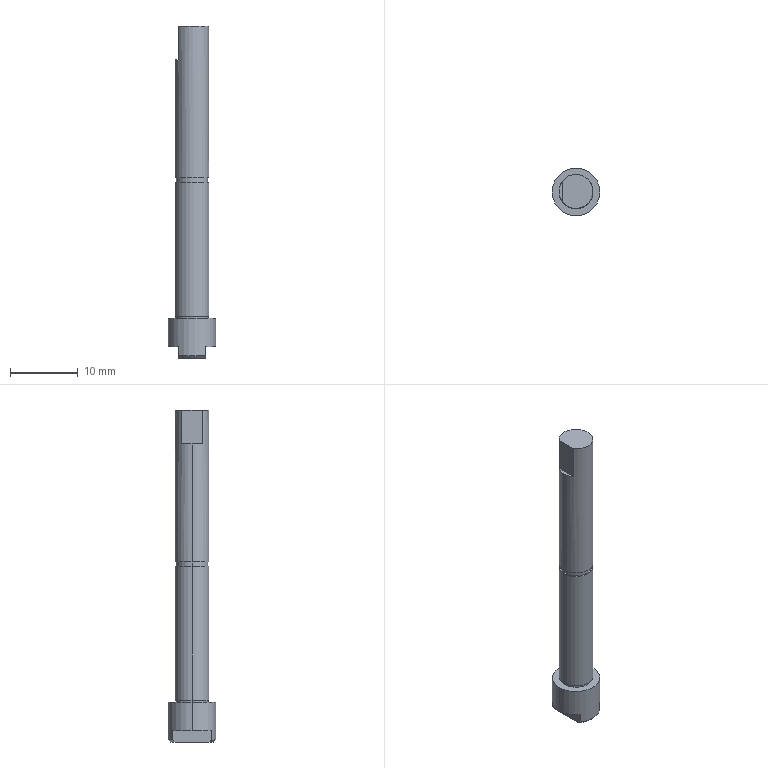Part | NX | 1 solid | 30 faces | box 7 x 7 x 48.83 mm | volume 994.875 mm3 | plane 12 | cylinder 12 | cone 6 | commonest cylinder face diameters 5 x4 2.5 x2 4.6 x2 4.8 x2 7 x2
STEP:
#1=CARTESIAN_POINT('',(-2.,1.5,43.));
#2=VERTEX_POINT('',#1);
#3=CARTESIAN_POINT('',(-2.,-1.5,43.));
#4=VERTEX_POINT('',#3);
#5=CARTESIAN_POINT('',(-2.,1.5,43.));
#6=DIRECTION('',(0.,-1.,0.));
#7=VECTOR('',#6,1000.);
#8=LINE('',#5,#7);
#9=EDGE_CURVE('',#2,#4,#8,.T.);
#10=ORIENTED_EDGE('',*,*,#9,.T.);
#11=CARTESIAN_POINT('',(2.5,0.,43.));
#12=VERTEX_POINT('',#11);
#13=CARTESIAN_POINT('',(0.,0.,43.));
#14=DIRECTION('',(0.,0.,-1.));
#15=DIRECTION('',(1.,0.,0.));
#16=AXIS2_PLACEMENT_3D('',#13,#14,#15);
#17=CIRCLE('',#16,2.5);
#18=EDGE_CURVE('',#12,#4,#17,.T.);
#19=ORIENTED_EDGE('',*,*,#18,.F.);
#20=CARTESIAN_POINT('',(0.,0.,43.));
#21=DIRECTION('',(0.,0.,-1.));
#22=DIRECTION('',(1.,0.,0.));
#23=AXIS2_PLACEMENT_3D('',#20,#21,#22);
#24=CIRCLE('',#23,2.5);
#25=EDGE_CURVE('',#2,#12,#24,.T.);
#26=ORIENTED_EDGE('',*,*,#25,.F.);
#27=EDGE_LOOP('',(#10,#19,#26));
#28=FACE_BOUND('',#27,.T.);
#29=CARTESIAN_POINT('',(0.,0.,43.));
#30=DIRECTION('',(0.,0.,1.));
#31=DIRECTION('',(1.,0.,0.));
#32=AXIS2_PLACEMENT_3D('',#29,#30,#31);
#33=PLANE('',#32);
#34=ADVANCED_FACE('',(#28),#33,.T.);
#35=ORIENTED_EDGE('',*,*,#9,.F.);
#36=CARTESIAN_POINT('',(-2.,1.5,38.));
#37=VERTEX_POINT('',#36);
#38=CARTESIAN_POINT('',(-2.,1.5,43.));
#39=DIRECTION('',(0.,0.,-1.));
#40=VECTOR('',#39,1000.);
#41=LINE('',#38,#40);
#42=EDGE_CURVE('',#2,#37,#41,.T.);
#43=ORIENTED_EDGE('',*,*,#42,.T.);
#44=CARTESIAN_POINT('',(-2.,-1.5,38.));
#45=VERTEX_POINT('',#44);
#46=CARTESIAN_POINT('',(-2.,1.5,38.));
#47=DIRECTION('',(0.,-1.,0.));
#48=VECTOR('',#47,1000.);
#49=LINE('',#46,#48);
#50=EDGE_CURVE('',#37,#45,#49,.T.);
#51=ORIENTED_EDGE('',*,*,#50,.T.);
#52=CARTESIAN_POINT('',(-2.,-1.5,38.));
#53=DIRECTION('',(0.,0.,1.));
#54=VECTOR('',#53,1000.);
#55=LINE('',#52,#54);
#56=EDGE_CURVE('',#45,#4,#55,.T.);
#57=ORIENTED_EDGE('',*,*,#56,.T.);
#58=EDGE_LOOP('',(#35,#43,#51,#57));
#59=FACE_BOUND('',#58,.T.);
#60=CARTESIAN_POINT('',(-2.,-3.316,43.));
#61=DIRECTION('',(1.,0.,0.));
#62=DIRECTION('',(0.,1.,0.));
#63=AXIS2_PLACEMENT_3D('',#60,#61,#62);
#64=PLANE('',#63);
#65=ADVANCED_FACE('',(#59),#64,.F.);
#66=CARTESIAN_POINT('',(-2.5,0.,38.));
#67=VERTEX_POINT('',#66);
#68=CARTESIAN_POINT('',(0.,0.,38.));
#69=DIRECTION('',(0.,0.,-1.));
#70=DIRECTION('',(-0.8,-0.6,0.));
#71=AXIS2_PLACEMENT_3D('',#68,#69,#70);
#72=CIRCLE('',#71,2.5);
#73=EDGE_CURVE('',#67,#37,#72,.T.);
#74=ORIENTED_EDGE('',*,*,#73,.T.);
#75=ORIENTED_EDGE('',*,*,#42,.F.);
#76=ORIENTED_EDGE('',*,*,#25,.T.);
#77=CARTESIAN_POINT('',(2.5,0.,20.65));
#78=VERTEX_POINT('',#77);
#79=CARTESIAN_POINT('',(2.5,0.,0.));
#80=DIRECTION('',(0.,0.,1.));
#81=VECTOR('',#80,1000.);
#82=LINE('',#79,#81);
#83=EDGE_CURVE('',#78,#12,#82,.T.);
#84=ORIENTED_EDGE('',*,*,#83,.F.);
#85=CARTESIAN_POINT('',(-2.5,0.,20.65));
#86=VERTEX_POINT('',#85);
#87=CARTESIAN_POINT('',(0.,0.,20.65));
#88=DIRECTION('',(0.,0.,1.));
#89=DIRECTION('',(1.,0.,0.));
#90=AXIS2_PLACEMENT_3D('',#87,#88,#89);
#91=CIRCLE('',#90,2.5);
#92=EDGE_CURVE('',#78,#86,#91,.T.);
#93=ORIENTED_EDGE('',*,*,#92,.T.);
#94=CARTESIAN_POINT('',(-2.5,0.,0.));
#95=DIRECTION('',(0.,0.,1.));
#96=VECTOR('',#95,1000.);
#97=LINE('',#94,#96);
#98=EDGE_CURVE('',#86,#67,#97,.T.);
#99=ORIENTED_EDGE('',*,*,#98,.T.);
#100=EDGE_LOOP('',(#74,#75,#76,#84,#93,#99));
#101=FACE_BOUND('',#100,.T.);
#102=CARTESIAN_POINT('',(0.,0.,0.));
#103=DIRECTION('',(0.,0.,1.));
#104=DIRECTION('',(1.,0.,0.));
#105=AXIS2_PLACEMENT_3D('',#102,#103,#104);
#106=CYLINDRICAL_SURFACE('',#105,2.5);
#107=ADVANCED_FACE('',(#101),#106,.T.);
#108=CARTESIAN_POINT('',(-2.,-2.498,-5.83));
#109=VERTEX_POINT('',#108);
#110=CARTESIAN_POINT('',(2.,-2.498,-5.83));
#111=VERTEX_POINT('',#110);
#112=CARTESIAN_POINT('',(0.,0.,-5.83));
#113=DIRECTION('',(0.,0.,1.));
#114=DIRECTION('',(1.,0.,0.));
#115=AXIS2_PLACEMENT_3D('',#112,#113,#114);
#116=CIRCLE('',#115,3.2);
#117=EDGE_CURVE('',#109,#111,#116,.T.);
#118=ORIENTED_EDGE('',*,*,#117,.T.);
#119=CARTESIAN_POINT('',(2.,-2.872,-5.53));
#120=VERTEX_POINT('',#119);
#121=CARTESIAN_POINT('',(2.,-2.872,-5.53));
#122=CARTESIAN_POINT('',(2.,-2.83,-5.565));
#123=CARTESIAN_POINT('',(2.,-2.745,-5.634));
#124=CARTESIAN_POINT('',(2.,-2.62,-5.734));
#125=CARTESIAN_POINT('',(2.,-2.539,-5.798));
#126=CARTESIAN_POINT('',(2.,-2.498,-5.83));
#127=B_SPLINE_CURVE_WITH_KNOTS('',3,(#121,#122,#123,#124,#125,#126),.UNSPECIFIED.,.F.,.F.,(4,1,1,4),(0.,0.3333,0.6667,1.),.UNSPECIFIED.);
#128=EDGE_CURVE('',#120,#111,#127,.T.);
#129=ORIENTED_EDGE('',*,*,#128,.F.);
#130=CARTESIAN_POINT('',(-2.,-2.872,-5.53));
#131=VERTEX_POINT('',#130);
#132=CARTESIAN_POINT('',(0.,0.,-5.53));
#133=DIRECTION('',(0.,0.,1.));
#134=DIRECTION('',(-0.5714,-0.8207,0.));
#135=AXIS2_PLACEMENT_3D('',#132,#133,#134);
#136=CIRCLE('',#135,3.5);
#137=EDGE_CURVE('',#131,#120,#136,.T.);
#138=ORIENTED_EDGE('',*,*,#137,.F.);
#139=CARTESIAN_POINT('',(-2.,-2.872,-5.53));
#140=CARTESIAN_POINT('',(-2.,-2.743,-5.636));
#141=CARTESIAN_POINT('',(-2.,-2.618,-5.736));
#142=CARTESIAN_POINT('',(-2.,-2.498,-5.83));
#143=B_SPLINE_CURVE_WITH_KNOTS('',3,(#139,#140,#141,#142),.UNSPECIFIED.,.F.,.F.,(4,4),(0.,1.),.UNSPECIFIED.);
#144=EDGE_CURVE('',#131,#109,#143,.T.);
#145=ORIENTED_EDGE('',*,*,#144,.T.);
#146=EDGE_LOOP('',(#118,#129,#138,#145));
#147=FACE_BOUND('',#146,.T.);
#148=CARTESIAN_POINT('',(0.,0.,-5.68));
#149=DIRECTION('',(0.,0.,1.));
#150=DIRECTION('',(1.,0.,0.));
#151=AXIS2_PLACEMENT_3D('',#148,#149,#150);
#152=CONICAL_SURFACE('',#151,3.35,0.7854);
#153=ADVANCED_FACE('',(#147),#152,.T.);
#154=ORIENTED_EDGE('',*,*,#73,.F.);
#155=CARTESIAN_POINT('',(0.,0.,38.));
#156=DIRECTION('',(0.,0.,-1.));
#157=DIRECTION('',(-0.8,-0.6,0.));
#158=AXIS2_PLACEMENT_3D('',#155,#156,#157);
#159=CIRCLE('',#158,2.5);
#160=EDGE_CURVE('',#45,#67,#159,.T.);
#161=ORIENTED_EDGE('',*,*,#160,.F.);
#162=ORIENTED_EDGE('',*,*,#50,.F.);
#163=EDGE_LOOP('',(#154,#161,#162));
#164=FACE_BOUND('',#163,.T.);
#165=CARTESIAN_POINT('',(0.,0.,38.));
#166=DIRECTION('',(0.,0.,1.));
#167=DIRECTION('',(1.,0.,0.));
#168=AXIS2_PLACEMENT_3D('',#165,#166,#167);
#169=PLANE('',#168);
#170=ADVANCED_FACE('',(#164),#169,.T.);
#171=ORIENTED_EDGE('',*,*,#92,.F.);
#172=CARTESIAN_POINT('',(0.,0.,20.65));
#173=DIRECTION('',(0.,0.,1.));
#174=DIRECTION('',(1.,0.,0.));
#175=AXIS2_PLACEMENT_3D('',#172,#173,#174);
#176=CIRCLE('',#175,2.5);
#177=EDGE_CURVE('',#86,#78,#176,.T.);
#178=ORIENTED_EDGE('',*,*,#177,.F.);
#179=EDGE_LOOP('',(#171,#178));
#180=FACE_BOUND('',#179,.T.);
#181=CARTESIAN_POINT('',(2.3,0.,20.65));
#182=VERTEX_POINT('',#181);
#183=CARTESIAN_POINT('',(-2.3,0.,20.65));
#184=VERTEX_POINT('',#183);
#185=CARTESIAN_POINT('',(0.,0.,20.65));
#186=DIRECTION('',(0.,0.,-1.));
#187=DIRECTION('',(1.,0.,0.));
#188=AXIS2_PLACEMENT_3D('',#185,#186,#187);
#189=CIRCLE('',#188,2.3);
#190=EDGE_CURVE('',#182,#184,#189,.T.);
#191=ORIENTED_EDGE('',*,*,#190,.F.);
#192=CARTESIAN_POINT('',(0.,0.,20.65));
#193=DIRECTION('',(0.,0.,-1.));
#194=DIRECTION('',(1.,0.,0.));
#195=AXIS2_PLACEMENT_3D('',#192,#193,#194);
#196=CIRCLE('',#195,2.3);
#197=EDGE_CURVE('',#184,#182,#196,.T.);
#198=ORIENTED_EDGE('',*,*,#197,.F.);
#199=EDGE_LOOP('',(#191,#198));
#200=FACE_BOUND('',#199,.T.);
#201=CARTESIAN_POINT('',(0.,0.,20.65));
#202=DIRECTION('',(0.,0.,-1.));
#203=DIRECTION('',(0.,-1.,0.));
#204=AXIS2_PLACEMENT_3D('',#201,#202,#203);
#205=PLANE('',#204);
#206=ADVANCED_FACE('',(#180,#200),#205,.T.);
#207=ORIENTED_EDGE('',*,*,#190,.T.);
#208=CARTESIAN_POINT('',(-2.3,0.,20.));
#209=VERTEX_POINT('',#208);
#210=CARTESIAN_POINT('',(-2.3,0.,20.683));
#211=DIRECTION('',(0.,0.,-1.));
#212=VECTOR('',#211,1000.);
#213=LINE('',#210,#212);
#214=EDGE_CURVE('',#209,#184,#213,.F.);
#215=ORIENTED_EDGE('',*,*,#214,.F.);
#216=CARTESIAN_POINT('',(2.3,0.,20.));
#217=VERTEX_POINT('',#216);
#218=CARTESIAN_POINT('',(0.,0.,20.));
#219=DIRECTION('',(0.,0.,1.));
#220=DIRECTION('',(1.,0.,0.));
#221=AXIS2_PLACEMENT_3D('',#218,#219,#220);
#222=CIRCLE('',#221,2.3);
#223=EDGE_CURVE('',#209,#217,#222,.T.);
#224=ORIENTED_EDGE('',*,*,#223,.T.);
#225=CARTESIAN_POINT('',(2.3,0.,20.683));
#226=DIRECTION('',(0.,0.,-1.));
#227=VECTOR('',#226,1000.);
#228=LINE('',#225,#227);
#229=EDGE_CURVE('',#217,#182,#228,.F.);
#230=ORIENTED_EDGE('',*,*,#229,.T.);
#231=EDGE_LOOP('',(#207,#215,#224,#230));
#232=FACE_BOUND('',#231,.T.);
#233=CARTESIAN_POINT('',(0.,0.,20.683));
#234=DIRECTION('',(0.,0.,-1.));
#235=DIRECTION('',(-1.,0.,0.));
#236=AXIS2_PLACEMENT_3D('',#233,#234,#235);
#237=CYLINDRICAL_SURFACE('',#236,2.3);
#238=ADVANCED_FACE('',(#232),#237,.T.);
#239=CARTESIAN_POINT('',(2.,2.498,-5.83));
#240=VERTEX_POINT('',#239);
#241=CARTESIAN_POINT('',(-2.,2.498,-5.83));
#242=VERTEX_POINT('',#241);
#243=CARTESIAN_POINT('',(0.,0.,-5.83));
#244=DIRECTION('',(0.,0.,1.));
#245=DIRECTION('',(1.,0.,0.));
#246=AXIS2_PLACEMENT_3D('',#243,#244,#245);
#247=CIRCLE('',#246,3.2);
#248=EDGE_CURVE('',#240,#242,#247,.T.);
#249=ORIENTED_EDGE('',*,*,#248,.T.);
#250=CARTESIAN_POINT('',(-2.,2.872,-5.53));
#251=VERTEX_POINT('',#250);
#252=CARTESIAN_POINT('',(-2.,2.872,-5.53));
#253=CARTESIAN_POINT('',(-2.,2.83,-5.565));
#254=CARTESIAN_POINT('',(-2.,2.745,-5.634));
#255=CARTESIAN_POINT('',(-2.,2.62,-5.734));
#256=CARTESIAN_POINT('',(-2.,2.539,-5.798));
#257=CARTESIAN_POINT('',(-2.,2.498,-5.83));
#258=B_SPLINE_CURVE_WITH_KNOTS('',3,(#252,#253,#254,#255,#256,#257),.UNSPECIFIED.,.F.,.F.,(4,1,1,4),(0.,0.3333,0.6667,1.),.UNSPECIFIED.);
#259=EDGE_CURVE('',#251,#242,#258,.T.);
#260=ORIENTED_EDGE('',*,*,#259,.F.);
#261=CARTESIAN_POINT('',(2.,2.872,-5.53));
#262=VERTEX_POINT('',#261);
#263=CARTESIAN_POINT('',(0.,0.,-5.53));
#264=DIRECTION('',(0.,0.,1.));
#265=DIRECTION('',(0.5714,0.8207,0.));
#266=AXIS2_PLACEMENT_3D('',#263,#264,#265);
#267=CIRCLE('',#266,3.5);
#268=EDGE_CURVE('',#262,#251,#267,.T.);
#269=ORIENTED_EDGE('',*,*,#268,.F.);
#270=CARTESIAN_POINT('',(2.,2.872,-5.53));
#271=CARTESIAN_POINT('',(2.,2.743,-5.636));
#272=CARTESIAN_POINT('',(2.,2.618,-5.736));
#273=CARTESIAN_POINT('',(2.,2.498,-5.83));
#274=B_SPLINE_CURVE_WITH_KNOTS('',3,(#270,#271,#272,#273),.UNSPECIFIED.,.F.,.F.,(4,4),(0.,1.),.UNSPECIFIED.);
#275=EDGE_CURVE('',#262,#240,#274,.T.);
#276=ORIENTED_EDGE('',*,*,#275,.T.);
#277=EDGE_LOOP('',(#249,#260,#269,#276));
#278=FACE_BOUND('',#277,.T.);
#279=CARTESIAN_POINT('',(0.,0.,-5.68));
#280=DIRECTION('',(0.,0.,1.));
#281=DIRECTION('',(1.,0.,0.));
#282=AXIS2_PLACEMENT_3D('',#279,#280,#281);
#283=CONICAL_SURFACE('',#282,3.35,0.7854);
#284=ADVANCED_FACE('',(#278),#283,.T.);
#285=CARTESIAN_POINT('',(-2.5,0.,20.));
#286=VERTEX_POINT('',#285);
#287=CARTESIAN_POINT('',(2.5,0.,20.));
#288=VERTEX_POINT('',#287);
#289=CARTESIAN_POINT('',(0.,0.,20.));
#290=DIRECTION('',(0.,0.,-1.));
#291=DIRECTION('',(1.,0.,0.));
#292=AXIS2_PLACEMENT_3D('',#289,#290,#291);
#293=CIRCLE('',#292,2.5);
#294=EDGE_CURVE('',#286,#288,#293,.T.);
#295=ORIENTED_EDGE('',*,*,#294,.F.);
#296=CARTESIAN_POINT('',(0.,0.,20.));
#297=DIRECTION('',(0.,0.,-1.));
#298=DIRECTION('',(1.,0.,0.));
#299=AXIS2_PLACEMENT_3D('',#296,#297,#298);
#300=CIRCLE('',#299,2.5);
#301=EDGE_CURVE('',#288,#286,#300,.T.);
#302=ORIENTED_EDGE('',*,*,#301,.F.);
#303=EDGE_LOOP('',(#295,#302));
#304=FACE_BOUND('',#303,.T.);
#305=CARTESIAN_POINT('',(0.,0.,20.));
#306=DIRECTION('',(0.,0.,1.));
#307=DIRECTION('',(1.,0.,0.));
#308=AXIS2_PLACEMENT_3D('',#305,#306,#307);
#309=CIRCLE('',#308,2.3);
#310=EDGE_CURVE('',#217,#209,#309,.T.);
#311=ORIENTED_EDGE('',*,*,#310,.F.);
#312=ORIENTED_EDGE('',*,*,#223,.F.);
#313=EDGE_LOOP('',(#311,#312));
#314=FACE_BOUND('',#313,.T.);
#315=CARTESIAN_POINT('',(0.,0.,20.));
#316=DIRECTION('',(0.,0.,-1.));
#317=DIRECTION('',(0.,-1.,0.));
#318=AXIS2_PLACEMENT_3D('',#315,#316,#317);
#319=PLANE('',#318);
#320=ADVANCED_FACE('',(#304,#314),#319,.F.);
#321=ORIENTED_EDGE('',*,*,#294,.T.);
#322=CARTESIAN_POINT('',(2.5,0.,0.3));
#323=VERTEX_POINT('',#322);
#324=CARTESIAN_POINT('',(2.5,0.,0.));
#325=DIRECTION('',(0.,0.,1.));
#326=VECTOR('',#325,1000.);
#327=LINE('',#324,#326);
#328=EDGE_CURVE('',#323,#288,#327,.T.);
#329=ORIENTED_EDGE('',*,*,#328,.F.);
#330=CARTESIAN_POINT('',(-2.5,0.,0.3));
#331=VERTEX_POINT('',#330);
#332=CARTESIAN_POINT('',(0.,0.,0.3));
#333=DIRECTION('',(0.,0.,1.));
#334=DIRECTION('',(-1.,0.,0.));
#335=AXIS2_PLACEMENT_3D('',#332,#333,#334);
#336=CIRCLE('',#335,2.5);
#337=EDGE_CURVE('',#323,#331,#336,.T.);
#338=ORIENTED_EDGE('',*,*,#337,.T.);
#339=CARTESIAN_POINT('',(-2.5,0.,0.));
#340=DIRECTION('',(0.,0.,1.));
#341=VECTOR('',#340,1000.);
#342=LINE('',#339,#341);
#343=EDGE_CURVE('',#331,#286,#342,.T.);
#344=ORIENTED_EDGE('',*,*,#343,.T.);
#345=EDGE_LOOP('',(#321,#329,#338,#344));
#346=FACE_BOUND('',#345,.T.);
#347=CARTESIAN_POINT('',(0.,0.,0.));
#348=DIRECTION('',(0.,0.,1.));
#349=DIRECTION('',(1.,0.,0.));
#350=AXIS2_PLACEMENT_3D('',#347,#348,#349);
#351=CYLINDRICAL_SURFACE('',#350,2.5);
#352=ADVANCED_FACE('',(#346),#351,.T.);
#353=CARTESIAN_POINT('',(0.,0.,0.3));
#354=DIRECTION('',(0.,0.,1.));
#355=DIRECTION('',(-1.,0.,0.));
#356=AXIS2_PLACEMENT_3D('',#353,#354,#355);
#357=CIRCLE('',#356,2.5);
#358=EDGE_CURVE('',#331,#323,#357,.T.);
#359=ORIENTED_EDGE('',*,*,#358,.F.);
#360=ORIENTED_EDGE('',*,*,#337,.F.);
#361=EDGE_LOOP('',(#359,#360));
#362=FACE_BOUND('',#361,.T.);
#363=CARTESIAN_POINT('',(2.4,0.,0.3));
#364=VERTEX_POINT('',#363);
#365=CARTESIAN_POINT('',(-2.4,0.,0.3));
#366=VERTEX_POINT('',#365);
#367=CARTESIAN_POINT('',(0.,0.,0.3));
#368=DIRECTION('',(0.,0.,-1.));
#369=DIRECTION('',(-1.,0.,0.));
#370=AXIS2_PLACEMENT_3D('',#367,#368,#369);
#371=CIRCLE('',#370,2.4);
#372=EDGE_CURVE('',#364,#366,#371,.T.);
#373=ORIENTED_EDGE('',*,*,#372,.F.);
#374=CARTESIAN_POINT('',(0.,0.,0.3));
#375=DIRECTION('',(0.,0.,-1.));
#376=DIRECTION('',(-1.,0.,0.));
#377=AXIS2_PLACEMENT_3D('',#374,#375,#376);
#378=CIRCLE('',#377,2.4);
#379=EDGE_CURVE('',#366,#364,#378,.T.);
#380=ORIENTED_EDGE('',*,*,#379,.F.);
#381=EDGE_LOOP('',(#373,#380));
#382=FACE_BOUND('',#381,.T.);
#383=CARTESIAN_POINT('',(0.,0.,0.3));
#384=DIRECTION('',(0.,0.,-1.));
#385=DIRECTION('',(0.,-1.,0.));
#386=AXIS2_PLACEMENT_3D('',#383,#384,#385);
#387=PLANE('',#386);
#388=ADVANCED_FACE('',(#362,#382),#387,.T.);
#389=CARTESIAN_POINT('',(2.,0.,-5.83));
#390=DIRECTION('',(0.,-1.,0.));
#391=VECTOR('',#390,1000.);
#392=LINE('',#389,#391);
#393=EDGE_CURVE('',#240,#111,#392,.T.);
#394=ORIENTED_EDGE('',*,*,#393,.F.);
#395=ORIENTED_EDGE('',*,*,#275,.F.);
#396=CARTESIAN_POINT('',(2.,2.872,-4.18));
#397=VERTEX_POINT('',#396);
#398=CARTESIAN_POINT('',(2.,2.872,-5.53));
#399=DIRECTION('',(0.000000407,-0.000000283,1.));
#400=VECTOR('',#399,1000.);
#401=LINE('',#398,#400);
#402=EDGE_CURVE('',#262,#397,#401,.T.);
#403=ORIENTED_EDGE('',*,*,#402,.T.);
#404=CARTESIAN_POINT('',(2.,-2.872,-4.18));
#405=VERTEX_POINT('',#404);
#406=CARTESIAN_POINT('',(2.,2.872,-4.18));
#407=DIRECTION('',(0.,-1.,0.));
#408=VECTOR('',#407,1000.);
#409=LINE('',#406,#408);
#410=EDGE_CURVE('',#397,#405,#409,.T.);
#411=ORIENTED_EDGE('',*,*,#410,.T.);
#412=CARTESIAN_POINT('',(2.,-2.872,-4.18));
#413=DIRECTION('',(-0.000000407,-0.000000283,-1.));
#414=VECTOR('',#413,1000.);
#415=LINE('',#412,#414);
#416=EDGE_CURVE('',#405,#120,#415,.T.);
#417=ORIENTED_EDGE('',*,*,#416,.T.);
#418=ORIENTED_EDGE('',*,*,#128,.T.);
#419=EDGE_LOOP('',(#394,#395,#403,#411,#417,#418));
#420=FACE_BOUND('',#419,.T.);
#421=CARTESIAN_POINT('',(2.,-2.872,-5.83));
#422=DIRECTION('',(-1.,0.,0.));
#423=DIRECTION('',(0.,0.,1.));
#424=AXIS2_PLACEMENT_3D('',#421,#422,#423);
#425=PLANE('',#424);
#426=ADVANCED_FACE('',(#420),#425,.F.);
#427=ORIENTED_EDGE('',*,*,#372,.T.);
#428=CARTESIAN_POINT('',(-2.4,0.,0.));
#429=VERTEX_POINT('',#428);
#430=CARTESIAN_POINT('',(-2.4,0.,0.315));
#431=DIRECTION('',(0.,0.,-1.));
#432=VECTOR('',#431,1000.);
#433=LINE('',#430,#432);
#434=EDGE_CURVE('',#366,#429,#433,.T.);
#435=ORIENTED_EDGE('',*,*,#434,.T.);
#436=CARTESIAN_POINT('',(2.4,0.,0.));
#437=VERTEX_POINT('',#436);
#438=CARTESIAN_POINT('',(0.,0.,0.));
#439=DIRECTION('',(0.,0.,1.));
#440=DIRECTION('',(1.,0.,0.));
#441=AXIS2_PLACEMENT_3D('',#438,#439,#440);
#442=CIRCLE('',#441,2.4);
#443=EDGE_CURVE('',#429,#437,#442,.T.);
#444=ORIENTED_EDGE('',*,*,#443,.T.);
#445=CARTESIAN_POINT('',(2.4,0.,0.315));
#446=DIRECTION('',(0.,0.,-1.));
#447=VECTOR('',#446,1000.);
#448=LINE('',#445,#447);
#449=EDGE_CURVE('',#364,#437,#448,.T.);
#450=ORIENTED_EDGE('',*,*,#449,.F.);
#451=EDGE_LOOP('',(#427,#435,#444,#450));
#452=FACE_BOUND('',#451,.T.);
#453=CARTESIAN_POINT('',(0.,0.,0.315));
#454=DIRECTION('',(0.,0.,-1.));
#455=DIRECTION('',(1.,0.,0.));
#456=AXIS2_PLACEMENT_3D('',#453,#454,#455);
#457=CYLINDRICAL_SURFACE('',#456,2.4);
#458=ADVANCED_FACE('',(#452),#457,.T.);
#459=CARTESIAN_POINT('',(-2.,0.,-5.83));
#460=DIRECTION('',(0.,1.,0.));
#461=VECTOR('',#460,1000.);
#462=LINE('',#459,#461);
#463=EDGE_CURVE('',#109,#242,#462,.T.);
#464=ORIENTED_EDGE('',*,*,#463,.F.);
#465=ORIENTED_EDGE('',*,*,#144,.F.);
#466=CARTESIAN_POINT('',(-2.,-2.872,-4.18));
#467=VERTEX_POINT('',#466);
#468=CARTESIAN_POINT('',(-2.,-2.872,-5.53));
#469=DIRECTION('',(-0.000000407,0.000000283,1.));
#470=VECTOR('',#469,1000.);
#471=LINE('',#468,#470);
#472=EDGE_CURVE('',#131,#467,#471,.T.);
#473=ORIENTED_EDGE('',*,*,#472,.T.);
#474=CARTESIAN_POINT('',(-2.,2.872,-4.18));
#475=VERTEX_POINT('',#474);
#476=CARTESIAN_POINT('',(-2.,-2.872,-4.18));
#477=DIRECTION('',(0.,1.,0.));
#478=VECTOR('',#477,1000.);
#479=LINE('',#476,#478);
#480=EDGE_CURVE('',#467,#475,#479,.T.);
#481=ORIENTED_EDGE('',*,*,#480,.T.);
#482=CARTESIAN_POINT('',(-2.,2.872,-4.18));
#483=DIRECTION('',(0.000000407,0.000000283,-1.));
#484=VECTOR('',#483,1000.);
#485=LINE('',#482,#484);
#486=EDGE_CURVE('',#475,#251,#485,.T.);
#487=ORIENTED_EDGE('',*,*,#486,.T.);
#488=ORIENTED_EDGE('',*,*,#259,.T.);
#489=EDGE_LOOP('',(#464,#465,#473,#481,#487,#488));
#490=FACE_BOUND('',#489,.T.);
#491=CARTESIAN_POINT('',(-2.,2.872,-5.83));
#492=DIRECTION('',(1.,0.,0.));
#493=DIRECTION('',(0.,1.,0.));
#494=AXIS2_PLACEMENT_3D('',#491,#492,#493);
#495=PLANE('',#494);
#496=ADVANCED_FACE('',(#490),#495,.F.);
#497=CARTESIAN_POINT('',(3.5,0.,0.));
#498=VERTEX_POINT('',#497);
#499=CARTESIAN_POINT('',(-3.5,0.,0.));
#500=VERTEX_POINT('',#499);
#501=CARTESIAN_POINT('',(0.,0.,0.));
#502=DIRECTION('',(0.,0.,-1.));
#503=DIRECTION('',(1.,0.,0.));
#504=AXIS2_PLACEMENT_3D('',#501,#502,#503);
#505=CIRCLE('',#504,3.5);
#506=EDGE_CURVE('',#498,#500,#505,.T.);
#507=ORIENTED_EDGE('',*,*,#506,.F.);
#508=CARTESIAN_POINT('',(0.,0.,0.));
#509=DIRECTION('',(0.,0.,-1.));
#510=DIRECTION('',(1.,0.,0.));
#511=AXIS2_PLACEMENT_3D('',#508,#509,#510);
#512=CIRCLE('',#511,3.5);
#513=EDGE_CURVE('',#500,#498,#512,.T.);
#514=ORIENTED_EDGE('',*,*,#513,.F.);
#515=EDGE_LOOP('',(#507,#514));
#516=FACE_BOUND('',#515,.T.);
#517=ORIENTED_EDGE('',*,*,#443,.F.);
#518=CARTESIAN_POINT('',(0.,0.,0.));
#519=DIRECTION('',(0.,0.,1.));
#520=DIRECTION('',(1.,0.,0.));
#521=AXIS2_PLACEMENT_3D('',#518,#519,#520);
#522=CIRCLE('',#521,2.4);
#523=EDGE_CURVE('',#437,#429,#522,.T.);
#524=ORIENTED_EDGE('',*,*,#523,.F.);
#525=EDGE_LOOP('',(#517,#524));
#526=FACE_BOUND('',#525,.T.);
#527=CARTESIAN_POINT('',(0.,0.,0.));
#528=DIRECTION('',(0.,0.,-1.));
#529=DIRECTION('',(0.,-1.,0.));
#530=AXIS2_PLACEMENT_3D('',#527,#528,#529);
#531=PLANE('',#530);
#532=ADVANCED_FACE('',(#516,#526),#531,.F.);
#533=CARTESIAN_POINT('',(-3.5,0.,-4.18));
#534=VERTEX_POINT('',#533);
#535=CARTESIAN_POINT('',(0.,0.,-4.18));
#536=DIRECTION('',(0.,0.,1.));
#537=DIRECTION('',(-1.,0.,0.));
#538=AXIS2_PLACEMENT_3D('',#535,#536,#537);
#539=CIRCLE('',#538,3.5);
#540=EDGE_CURVE('',#534,#467,#539,.T.);
#541=ORIENTED_EDGE('',*,*,#540,.T.);
#542=ORIENTED_EDGE('',*,*,#472,.F.);
#543=ORIENTED_EDGE('',*,*,#137,.T.);
#544=ORIENTED_EDGE('',*,*,#416,.F.);
#545=CARTESIAN_POINT('',(3.5,0.,-4.18));
#546=VERTEX_POINT('',#545);
#547=CARTESIAN_POINT('',(0.,0.,-4.18));
#548=DIRECTION('',(0.,0.,1.));
#549=DIRECTION('',(0.5714,-0.8207,0.));
#550=AXIS2_PLACEMENT_3D('',#547,#548,#549);
#551=CIRCLE('',#550,3.5);
#552=EDGE_CURVE('',#405,#546,#551,.T.);
#553=ORIENTED_EDGE('',*,*,#552,.T.);
#554=CARTESIAN_POINT('',(3.5,0.,0.));
#555=DIRECTION('',(0.,0.,-1.));
#556=VECTOR('',#555,1000.);
#557=LINE('',#554,#556);
#558=EDGE_CURVE('',#546,#498,#557,.F.);
#559=ORIENTED_EDGE('',*,*,#558,.T.);
#560=ORIENTED_EDGE('',*,*,#506,.T.);
#561=CARTESIAN_POINT('',(-3.5,0.,0.));
#562=DIRECTION('',(0.,0.,-1.));
#563=VECTOR('',#562,1000.);
#564=LINE('',#561,#563);
#565=EDGE_CURVE('',#534,#500,#564,.F.);
#566=ORIENTED_EDGE('',*,*,#565,.F.);
#567=EDGE_LOOP('',(#541,#542,#543,#544,#553,#559,#560,#566));
#568=FACE_BOUND('',#567,.T.);
#569=CARTESIAN_POINT('',(0.,0.,0.));
#570=DIRECTION('',(0.,0.,-1.));
#571=DIRECTION('',(-1.,0.,0.));
#572=AXIS2_PLACEMENT_3D('',#569,#570,#571);
#573=CYLINDRICAL_SURFACE('',#572,3.5);
#574=ADVANCED_FACE('',(#568),#573,.T.);
#575=ORIENTED_EDGE('',*,*,#540,.F.);
#576=CARTESIAN_POINT('',(0.,0.,-4.18));
#577=DIRECTION('',(0.,0.,1.));
#578=DIRECTION('',(-1.,0.,0.));
#579=AXIS2_PLACEMENT_3D('',#576,#577,#578);
#580=CIRCLE('',#579,3.5);
#581=EDGE_CURVE('',#475,#534,#580,.T.);
#582=ORIENTED_EDGE('',*,*,#581,.F.);
#583=ORIENTED_EDGE('',*,*,#480,.F.);
#584=EDGE_LOOP('',(#575,#582,#583));
#585=FACE_BOUND('',#584,.T.);
#586=CARTESIAN_POINT('',(0.,0.,-4.18));
#587=DIRECTION('',(0.,0.,-1.));
#588=DIRECTION('',(0.,-1.,0.));
#589=AXIS2_PLACEMENT_3D('',#586,#587,#588);
#590=PLANE('',#589);
#591=ADVANCED_FACE('',(#585),#590,.T.);
#592=ORIENTED_EDGE('',*,*,#393,.T.);
#593=ORIENTED_EDGE('',*,*,#117,.F.);
#594=ORIENTED_EDGE('',*,*,#463,.T.);
#595=ORIENTED_EDGE('',*,*,#248,.F.);
#596=EDGE_LOOP('',(#592,#593,#594,#595));
#597=FACE_BOUND('',#596,.T.);
#598=CARTESIAN_POINT('',(1.7,0.,-5.83));
#599=VERTEX_POINT('',#598);
#600=CARTESIAN_POINT('',(-1.7,0.,-5.83));
#601=VERTEX_POINT('',#600);
#602=CARTESIAN_POINT('',(0.,0.,-5.83));
#603=DIRECTION('',(0.,0.,-1.));
#604=DIRECTION('',(-1.,0.,0.));
#605=AXIS2_PLACEMENT_3D('',#602,#603,#604);
#606=CIRCLE('',#605,1.7);
#607=EDGE_CURVE('',#599,#601,#606,.T.);
#608=ORIENTED_EDGE('',*,*,#607,.F.);
#609=CARTESIAN_POINT('',(0.,0.,-5.83));
#610=DIRECTION('',(0.,0.,-1.));
#611=DIRECTION('',(-1.,0.,0.));
#612=AXIS2_PLACEMENT_3D('',#609,#610,#611);
#613=CIRCLE('',#612,1.7);
#614=EDGE_CURVE('',#601,#599,#613,.T.);
#615=ORIENTED_EDGE('',*,*,#614,.F.);
#616=EDGE_LOOP('',(#608,#615));
#617=FACE_BOUND('',#616,.T.);
#618=CARTESIAN_POINT('',(0.,0.,-5.83));
#619=DIRECTION('',(0.,0.,-1.));
#620=DIRECTION('',(0.,-1.,0.));
#621=AXIS2_PLACEMENT_3D('',#618,#619,#620);
#622=PLANE('',#621);
#623=ADVANCED_FACE('',(#597,#617),#622,.T.);
#624=CARTESIAN_POINT('',(0.,0.,-4.18));
#625=DIRECTION('',(0.,0.,1.));
#626=DIRECTION('',(0.5714,-0.8207,0.));
#627=AXIS2_PLACEMENT_3D('',#624,#625,#626);
#628=CIRCLE('',#627,3.5);
#629=EDGE_CURVE('',#546,#397,#628,.T.);
#630=ORIENTED_EDGE('',*,*,#629,.F.);
#631=ORIENTED_EDGE('',*,*,#552,.F.);
#632=ORIENTED_EDGE('',*,*,#410,.F.);
#633=EDGE_LOOP('',(#630,#631,#632));
#634=FACE_BOUND('',#633,.T.);
#635=CARTESIAN_POINT('',(0.,0.,-4.18));
#636=DIRECTION('',(0.,0.,-1.));
#637=DIRECTION('',(0.,-1.,0.));
#638=AXIS2_PLACEMENT_3D('',#635,#636,#637);
#639=PLANE('',#638);
#640=ADVANCED_FACE('',(#634),#639,.T.);
#641=CARTESIAN_POINT('',(-1.25,0.,-5.57));
#642=VERTEX_POINT('',#641);
#643=CARTESIAN_POINT('',(0.,1.25,-5.57));
#644=VERTEX_POINT('',#643);
#645=CARTESIAN_POINT('',(0.,0.,-5.57));
#646=DIRECTION('',(0.,0.,-1.));
#647=DIRECTION('',(-1.,0.,0.));
#648=AXIS2_PLACEMENT_3D('',#645,#646,#647);
#649=CIRCLE('',#648,1.25);
#650=EDGE_CURVE('',#642,#644,#649,.T.);
#651=ORIENTED_EDGE('',*,*,#650,.T.);
#652=CARTESIAN_POINT('',(0.,1.25,3.17));
#653=VERTEX_POINT('',#652);
#654=CARTESIAN_POINT('',(0.,1.25,-2.83));
#655=DIRECTION('',(0.,0.,-1.));
#656=VECTOR('',#655,1000.);
#657=LINE('',#654,#656);
#658=EDGE_CURVE('',#653,#644,#657,.T.);
#659=ORIENTED_EDGE('',*,*,#658,.F.);
#660=CARTESIAN_POINT('',(-1.25,0.,3.17));
#661=VERTEX_POINT('',#660);
#662=CARTESIAN_POINT('',(0.,0.,3.17));
#663=DIRECTION('',(0.,0.,1.));
#664=DIRECTION('',(1.,0.,0.));
#665=AXIS2_PLACEMENT_3D('',#662,#663,#664);
#666=CIRCLE('',#665,1.25);
#667=EDGE_CURVE('',#653,#661,#666,.T.);
#668=ORIENTED_EDGE('',*,*,#667,.T.);
#669=CARTESIAN_POINT('',(0.,-1.25,3.17));
#670=VERTEX_POINT('',#669);
#671=CARTESIAN_POINT('',(0.,0.,3.17));
#672=DIRECTION('',(0.,0.,1.));
#673=DIRECTION('',(1.,0.,0.));
#674=AXIS2_PLACEMENT_3D('',#671,#672,#673);
#675=CIRCLE('',#674,1.25);
#676=EDGE_CURVE('',#661,#670,#675,.T.);
#677=ORIENTED_EDGE('',*,*,#676,.T.);
#678=CARTESIAN_POINT('',(0.,-1.25,-5.57));
#679=VERTEX_POINT('',#678);
#680=CARTESIAN_POINT('',(0.,-1.25,-2.83));
#681=DIRECTION('',(0.,0.,-1.));
#682=VECTOR('',#681,1000.);
#683=LINE('',#680,#682);
#684=EDGE_CURVE('',#670,#679,#683,.T.);
#685=ORIENTED_EDGE('',*,*,#684,.T.);
#686=CARTESIAN_POINT('',(0.,0.,-5.57));
#687=DIRECTION('',(0.,0.,-1.));
#688=DIRECTION('',(-1.,0.,0.));
#689=AXIS2_PLACEMENT_3D('',#686,#687,#688);
#690=CIRCLE('',#689,1.25);
#691=EDGE_CURVE('',#679,#642,#690,.T.);
#692=ORIENTED_EDGE('',*,*,#691,.T.);
#693=EDGE_LOOP('',(#651,#659,#668,#677,#685,#692));
#694=FACE_BOUND('',#693,.T.);
#695=CARTESIAN_POINT('',(0.,0.,-2.83));
#696=DIRECTION('',(0.,0.,-1.));
#697=DIRECTION('',(0.,1.,0.));
#698=AXIS2_PLACEMENT_3D('',#695,#696,#697);
#699=CYLINDRICAL_SURFACE('',#698,1.25);
#700=ADVANCED_FACE('',(#694),#699,.F.);
#701=ORIENTED_EDGE('',*,*,#650,.F.);
#702=CARTESIAN_POINT('',(-1.25,0.,-5.57));
#703=DIRECTION('',(-0.866,0.,-0.5));
#704=VECTOR('',#703,1000.);
#705=LINE('',#702,#704);
#706=EDGE_CURVE('',#601,#642,#705,.F.);
#707=ORIENTED_EDGE('',*,*,#706,.F.);
#708=ORIENTED_EDGE('',*,*,#614,.T.);
#709=CARTESIAN_POINT('',(1.25,0.,-5.57));
#710=VERTEX_POINT('',#709);
#711=CARTESIAN_POINT('',(1.25,0.,-5.57));
#712=DIRECTION('',(0.866,0.,-0.5));
#713=VECTOR('',#712,1000.);
#714=LINE('',#711,#713);
#715=EDGE_CURVE('',#599,#710,#714,.F.);
#716=ORIENTED_EDGE('',*,*,#715,.T.);
#717=CARTESIAN_POINT('',(0.,0.,-5.57));
#718=DIRECTION('',(0.,0.,-1.));
#719=DIRECTION('',(-1.,0.,0.));
#720=AXIS2_PLACEMENT_3D('',#717,#718,#719);
#721=CIRCLE('',#720,1.25);
#722=EDGE_CURVE('',#644,#710,#721,.T.);
#723=ORIENTED_EDGE('',*,*,#722,.F.);
#724=EDGE_LOOP('',(#701,#707,#708,#716,#723));
#725=FACE_BOUND('',#724,.T.);
#726=CARTESIAN_POINT('',(0.,0.,-5.57));
#727=DIRECTION('',(0.,0.,-1.));
#728=DIRECTION('',(-1.,0.,0.));
#729=AXIS2_PLACEMENT_3D('',#726,#727,#728);
#730=CONICAL_SURFACE('',#729,1.25,1.047);
#731=ADVANCED_FACE('',(#725),#730,.F.);
#732=CARTESIAN_POINT('',(1.25,0.,3.17));
#733=VERTEX_POINT('',#732);
#734=CARTESIAN_POINT('',(0.,0.,3.17));
#735=DIRECTION('',(0.,0.,1.));
#736=DIRECTION('',(1.,0.,0.));
#737=AXIS2_PLACEMENT_3D('',#734,#735,#736);
#738=CIRCLE('',#737,1.25);
#739=EDGE_CURVE('',#733,#653,#738,.T.);
#740=ORIENTED_EDGE('',*,*,#739,.F.);
#741=CARTESIAN_POINT('',(0.,0.,3.921));
#742=VERTEX_POINT('',#741);
#743=CARTESIAN_POINT('',(1.25,0.,3.17));
#744=DIRECTION('',(0.8572,0.,-0.515));
#745=VECTOR('',#744,1000.);
#746=LINE('',#743,#745);
#747=EDGE_CURVE('',#742,#733,#746,.T.);
#748=ORIENTED_EDGE('',*,*,#747,.F.);
#749=CARTESIAN_POINT('',(-1.25,0.,3.17));
#750=DIRECTION('',(-0.8572,0.,-0.515));
#751=VECTOR('',#750,1000.);
#752=LINE('',#749,#751);
#753=EDGE_CURVE('',#742,#661,#752,.T.);
#754=ORIENTED_EDGE('',*,*,#753,.T.);
#755=ORIENTED_EDGE('',*,*,#667,.F.);
#756=EDGE_LOOP('',(#740,#748,#754,#755));
#757=FACE_BOUND('',#756,.T.);
#758=CARTESIAN_POINT('',(0.,0.,3.17));
#759=DIRECTION('',(0.,0.,-1.));
#760=DIRECTION('',(-1.,0.,0.));
#761=AXIS2_PLACEMENT_3D('',#758,#759,#760);
#762=CONICAL_SURFACE('',#761,1.25,1.03);
#763=ADVANCED_FACE('',(#757),#762,.F.);
#764=ORIENTED_EDGE('',*,*,#449,.T.);
#765=ORIENTED_EDGE('',*,*,#523,.T.);
#766=ORIENTED_EDGE('',*,*,#434,.F.);
#767=ORIENTED_EDGE('',*,*,#379,.T.);
#768=EDGE_LOOP('',(#764,#765,#766,#767));
#769=FACE_BOUND('',#768,.T.);
#770=CARTESIAN_POINT('',(0.,0.,0.315));
#771=DIRECTION('',(0.,0.,-1.));
#772=DIRECTION('',(1.,0.,0.));
#773=AXIS2_PLACEMENT_3D('',#770,#771,#772);
#774=CYLINDRICAL_SURFACE('',#773,2.4);
#775=ADVANCED_FACE('',(#769),#774,.T.);
#776=ORIENTED_EDGE('',*,*,#83,.T.);
#777=ORIENTED_EDGE('',*,*,#18,.T.);
#778=ORIENTED_EDGE('',*,*,#56,.F.);
#779=ORIENTED_EDGE('',*,*,#160,.T.);
#780=ORIENTED_EDGE('',*,*,#98,.F.);
#781=ORIENTED_EDGE('',*,*,#177,.T.);
#782=EDGE_LOOP('',(#776,#777,#778,#779,#780,#781));
#783=FACE_BOUND('',#782,.T.);
#784=CARTESIAN_POINT('',(0.,0.,0.));
#785=DIRECTION('',(0.,0.,1.));
#786=DIRECTION('',(1.,0.,0.));
#787=AXIS2_PLACEMENT_3D('',#784,#785,#786);
#788=CYLINDRICAL_SURFACE('',#787,2.5);
#789=ADVANCED_FACE('',(#783),#788,.T.);
#790=ORIENTED_EDGE('',*,*,#747,.T.);
#791=CARTESIAN_POINT('',(0.,0.,3.17));
#792=DIRECTION('',(0.,0.,1.));
#793=DIRECTION('',(1.,0.,0.));
#794=AXIS2_PLACEMENT_3D('',#791,#792,#793);
#795=CIRCLE('',#794,1.25);
#796=EDGE_CURVE('',#670,#733,#795,.T.);
#797=ORIENTED_EDGE('',*,*,#796,.F.);
#798=ORIENTED_EDGE('',*,*,#676,.F.);
#799=ORIENTED_EDGE('',*,*,#753,.F.);
#800=EDGE_LOOP('',(#790,#797,#798,#799));
#801=FACE_BOUND('',#800,.T.);
#802=CARTESIAN_POINT('',(0.,0.,3.17));
#803=DIRECTION('',(0.,0.,-1.));
#804=DIRECTION('',(-1.,0.,0.));
#805=AXIS2_PLACEMENT_3D('',#802,#803,#804);
#806=CONICAL_SURFACE('',#805,1.25,1.03);
#807=ADVANCED_FACE('',(#801),#806,.F.);
#808=ORIENTED_EDGE('',*,*,#358,.T.);
#809=ORIENTED_EDGE('',*,*,#328,.T.);
#810=ORIENTED_EDGE('',*,*,#301,.T.);
#811=ORIENTED_EDGE('',*,*,#343,.F.);
#812=EDGE_LOOP('',(#808,#809,#810,#811));
#813=FACE_BOUND('',#812,.T.);
#814=CARTESIAN_POINT('',(0.,0.,0.));
#815=DIRECTION('',(0.,0.,1.));
#816=DIRECTION('',(1.,0.,0.));
#817=AXIS2_PLACEMENT_3D('',#814,#815,#816);
#818=CYLINDRICAL_SURFACE('',#817,2.5);
#819=ADVANCED_FACE('',(#813),#818,.T.);
#820=ORIENTED_EDGE('',*,*,#607,.T.);
#821=ORIENTED_EDGE('',*,*,#706,.T.);
#822=ORIENTED_EDGE('',*,*,#691,.F.);
#823=CARTESIAN_POINT('',(0.,0.,-5.57));
#824=DIRECTION('',(0.,0.,-1.));
#825=DIRECTION('',(-1.,0.,0.));
#826=AXIS2_PLACEMENT_3D('',#823,#824,#825);
#827=CIRCLE('',#826,1.25);
#828=EDGE_CURVE('',#710,#679,#827,.T.);
#829=ORIENTED_EDGE('',*,*,#828,.F.);
#830=ORIENTED_EDGE('',*,*,#715,.F.);
#831=EDGE_LOOP('',(#820,#821,#822,#829,#830));
#832=FACE_BOUND('',#831,.T.);
#833=CARTESIAN_POINT('',(0.,0.,-5.57));
#834=DIRECTION('',(0.,0.,-1.));
#835=DIRECTION('',(-1.,0.,0.));
#836=AXIS2_PLACEMENT_3D('',#833,#834,#835);
#837=CONICAL_SURFACE('',#836,1.25,1.047);
#838=ADVANCED_FACE('',(#832),#837,.F.);
#839=ORIENTED_EDGE('',*,*,#565,.T.);
#840=ORIENTED_EDGE('',*,*,#513,.T.);
#841=ORIENTED_EDGE('',*,*,#558,.F.);
#842=ORIENTED_EDGE('',*,*,#629,.T.);
#843=ORIENTED_EDGE('',*,*,#402,.F.);
#844=ORIENTED_EDGE('',*,*,#268,.T.);
#845=ORIENTED_EDGE('',*,*,#486,.F.);
#846=ORIENTED_EDGE('',*,*,#581,.T.);
#847=EDGE_LOOP('',(#839,#840,#841,#842,#843,#844,#845,#846));
#848=FACE_BOUND('',#847,.T.);
#849=CARTESIAN_POINT('',(0.,0.,0.));
#850=DIRECTION('',(0.,0.,-1.));
#851=DIRECTION('',(-1.,0.,0.));
#852=AXIS2_PLACEMENT_3D('',#849,#850,#851);
#853=CYLINDRICAL_SURFACE('',#852,3.5);
#854=ADVANCED_FACE('',(#848),#853,.T.);
#855=ORIENTED_EDGE('',*,*,#310,.T.);
#856=ORIENTED_EDGE('',*,*,#214,.T.);
#857=ORIENTED_EDGE('',*,*,#197,.T.);
#858=ORIENTED_EDGE('',*,*,#229,.F.);
#859=EDGE_LOOP('',(#855,#856,#857,#858));
#860=FACE_BOUND('',#859,.T.);
#861=CARTESIAN_POINT('',(0.,0.,20.683));
#862=DIRECTION('',(0.,0.,-1.));
#863=DIRECTION('',(-1.,0.,0.));
#864=AXIS2_PLACEMENT_3D('',#861,#862,#863);
#865=CYLINDRICAL_SURFACE('',#864,2.3);
#866=ADVANCED_FACE('',(#860),#865,.T.);
#867=ORIENTED_EDGE('',*,*,#739,.T.);
#868=ORIENTED_EDGE('',*,*,#658,.T.);
#869=ORIENTED_EDGE('',*,*,#722,.T.);
#870=ORIENTED_EDGE('',*,*,#828,.T.);
#871=ORIENTED_EDGE('',*,*,#684,.F.);
#872=ORIENTED_EDGE('',*,*,#796,.T.);
#873=EDGE_LOOP('',(#867,#868,#869,#870,#871,#872));
#874=FACE_BOUND('',#873,.T.);
#875=CARTESIAN_POINT('',(0.,0.,-2.83));
#876=DIRECTION('',(0.,0.,-1.));
#877=DIRECTION('',(0.,1.,0.));
#878=AXIS2_PLACEMENT_3D('',#875,#876,#877);
#879=CYLINDRICAL_SURFACE('',#878,1.25);
#880=ADVANCED_FACE('',(#874),#879,.F.);
#881=CLOSED_SHELL('',(#34,#65,#107,#153,#170,#206,#238,#284,#320,#352,#388,#426,#458,#496,#532,#574,#591,#623,#640,#700,#731,#763,#775,#789,#807,#819,#838,#854,#866,#880));
#882=MANIFOLD_SOLID_BREP('',#881);
#883=(LENGTH_UNIT()NAMED_UNIT(*)SI_UNIT(.MILLI.,.METRE.));
#884=UNCERTAINTY_MEASURE_WITH_UNIT(LENGTH_MEASURE(0.00001),#883,'','');
#885=(NAMED_UNIT(*)PLANE_ANGLE_UNIT()SI_UNIT($,.RADIAN.));
#886=(NAMED_UNIT(*)SI_UNIT($,.STERADIAN.)SOLID_ANGLE_UNIT());
#887=(GEOMETRIC_REPRESENTATION_CONTEXT(3)GLOBAL_UNCERTAINTY_ASSIGNED_CONTEXT((#884))GLOBAL_UNIT_ASSIGNED_CONTEXT((#883,#885,#886))REPRESENTATION_CONTEXT('',''));
#888=ADVANCED_BREP_SHAPE_REPRESENTATION('',(#882),#887);